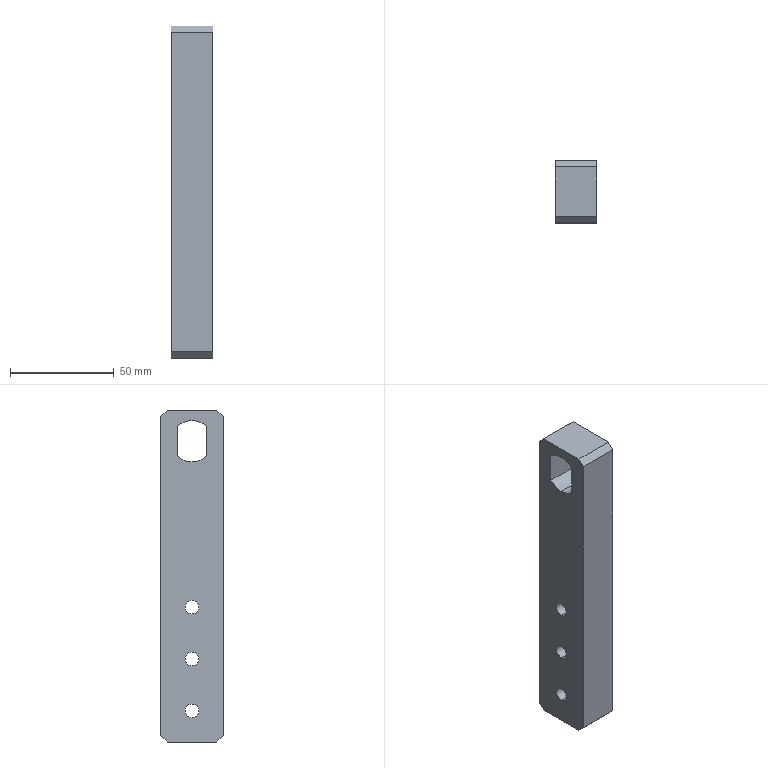Part | SolidWorks | features Chamfer 1, Extrusion 1, HoleWzd 1, ICE 1 | 1 solid | 30 faces | box 20 x 30 x 160 mm | volume 87200 mm3 | cylinder 15 | plane 15 | commonest cylinder face diameters 6.6 x6 11 x6 20 x3
STEP:
#1=CARTESIAN_POINT('',(13.2,0.,-9.5));
#2=VERTEX_POINT('',#1);
#3=CARTESIAN_POINT('',(13.2,0.,-20.5));
#4=VERTEX_POINT('',#3);
#5=CARTESIAN_POINT('',(13.2,0.,-15.));
#6=DIRECTION('',(1.,0.,0.));
#7=DIRECTION('',(0.,0.,-1.));
#8=AXIS2_PLACEMENT_3D('',#5,#6,#7);
#9=CIRCLE('',#8,5.5);
#10=EDGE_CURVE('',#2,#4,#9,.T.);
#11=ORIENTED_EDGE('',*,*,#10,.F.);
#12=CARTESIAN_POINT('',(20.,0.,-9.5));
#13=VERTEX_POINT('',#12);
#14=CARTESIAN_POINT('',(20.,0.,-9.5));
#15=DIRECTION('',(1.,0.,0.));
#16=VECTOR('',#15,1000.);
#17=LINE('',#14,#16);
#18=EDGE_CURVE('',#2,#13,#17,.T.);
#19=ORIENTED_EDGE('',*,*,#18,.T.);
#20=CARTESIAN_POINT('',(20.,0.,-20.5));
#21=VERTEX_POINT('',#20);
#22=CARTESIAN_POINT('',(20.,0.,-15.));
#23=DIRECTION('',(1.,0.,0.));
#24=DIRECTION('',(0.,0.,-1.));
#25=AXIS2_PLACEMENT_3D('',#22,#23,#24);
#26=CIRCLE('',#25,5.5);
#27=EDGE_CURVE('',#13,#21,#26,.T.);
#28=ORIENTED_EDGE('',*,*,#27,.T.);
#29=CARTESIAN_POINT('',(20.,0.,-20.5));
#30=DIRECTION('',(1.,0.,0.));
#31=VECTOR('',#30,1000.);
#32=LINE('',#29,#31);
#33=EDGE_CURVE('',#4,#21,#32,.T.);
#34=ORIENTED_EDGE('',*,*,#33,.F.);
#35=EDGE_LOOP('',(#11,#19,#28,#34));
#36=FACE_OUTER_BOUND('',#35,.T.);
#37=CARTESIAN_POINT('',(20.,0.,-15.));
#38=DIRECTION('',(1.,0.,0.));
#39=DIRECTION('',(0.,0.,-1.));
#40=AXIS2_PLACEMENT_3D('',#37,#38,#39);
#41=CYLINDRICAL_SURFACE('',#40,5.5);
#42=ADVANCED_FACE('',(#36),#41,.F.);
#43=CARTESIAN_POINT('',(0.,0.,-11.7));
#44=VERTEX_POINT('',#43);
#45=CARTESIAN_POINT('',(0.,0.,-18.3));
#46=VERTEX_POINT('',#45);
#47=CARTESIAN_POINT('',(0.,0.,-15.));
#48=DIRECTION('',(1.,0.,0.));
#49=DIRECTION('',(0.,0.,-1.));
#50=AXIS2_PLACEMENT_3D('',#47,#48,#49);
#51=CIRCLE('',#50,3.3);
#52=EDGE_CURVE('',#44,#46,#51,.T.);
#53=ORIENTED_EDGE('',*,*,#52,.F.);
#54=CARTESIAN_POINT('',(13.2,0.,-11.7));
#55=VERTEX_POINT('',#54);
#56=CARTESIAN_POINT('',(20.,0.,-11.7));
#57=DIRECTION('',(1.,0.,0.));
#58=VECTOR('',#57,1000.);
#59=LINE('',#56,#58);
#60=EDGE_CURVE('',#44,#55,#59,.T.);
#61=ORIENTED_EDGE('',*,*,#60,.T.);
#62=CARTESIAN_POINT('',(13.2,0.,-18.3));
#63=VERTEX_POINT('',#62);
#64=CARTESIAN_POINT('',(13.2,0.,-15.));
#65=DIRECTION('',(1.,0.,0.));
#66=DIRECTION('',(0.,0.,-1.));
#67=AXIS2_PLACEMENT_3D('',#64,#65,#66);
#68=CIRCLE('',#67,3.3);
#69=EDGE_CURVE('',#55,#63,#68,.T.);
#70=ORIENTED_EDGE('',*,*,#69,.T.);
#71=CARTESIAN_POINT('',(20.,0.,-18.3));
#72=DIRECTION('',(1.,0.,0.));
#73=VECTOR('',#72,1000.);
#74=LINE('',#71,#73);
#75=EDGE_CURVE('',#46,#63,#74,.T.);
#76=ORIENTED_EDGE('',*,*,#75,.F.);
#77=EDGE_LOOP('',(#53,#61,#70,#76));
#78=FACE_OUTER_BOUND('',#77,.T.);
#79=CARTESIAN_POINT('',(20.,0.,-15.));
#80=DIRECTION('',(1.,0.,0.));
#81=DIRECTION('',(0.,0.,-1.));
#82=AXIS2_PLACEMENT_3D('',#79,#80,#81);
#83=CYLINDRICAL_SURFACE('',#82,3.3);
#84=ADVANCED_FACE('',(#78),#83,.F.);
#85=CARTESIAN_POINT('',(13.2,0.,-34.5));
#86=VERTEX_POINT('',#85);
#87=CARTESIAN_POINT('',(13.2,0.,-45.5));
#88=VERTEX_POINT('',#87);
#89=CARTESIAN_POINT('',(13.2,0.,-40.));
#90=DIRECTION('',(1.,0.,0.));
#91=DIRECTION('',(0.,0.,-1.));
#92=AXIS2_PLACEMENT_3D('',#89,#90,#91);
#93=CIRCLE('',#92,5.5);
#94=EDGE_CURVE('',#86,#88,#93,.T.);
#95=ORIENTED_EDGE('',*,*,#94,.F.);
#96=CARTESIAN_POINT('',(20.,0.,-34.5));
#97=VERTEX_POINT('',#96);
#98=CARTESIAN_POINT('',(20.,0.,-34.5));
#99=DIRECTION('',(1.,0.,0.));
#100=VECTOR('',#99,1000.);
#101=LINE('',#98,#100);
#102=EDGE_CURVE('',#86,#97,#101,.T.);
#103=ORIENTED_EDGE('',*,*,#102,.T.);
#104=CARTESIAN_POINT('',(20.,0.,-45.5));
#105=VERTEX_POINT('',#104);
#106=CARTESIAN_POINT('',(20.,0.,-40.));
#107=DIRECTION('',(1.,0.,0.));
#108=DIRECTION('',(0.,0.,-1.));
#109=AXIS2_PLACEMENT_3D('',#106,#107,#108);
#110=CIRCLE('',#109,5.5);
#111=EDGE_CURVE('',#97,#105,#110,.T.);
#112=ORIENTED_EDGE('',*,*,#111,.T.);
#113=CARTESIAN_POINT('',(20.,0.,-45.5));
#114=DIRECTION('',(1.,0.,0.));
#115=VECTOR('',#114,1000.);
#116=LINE('',#113,#115);
#117=EDGE_CURVE('',#88,#105,#116,.T.);
#118=ORIENTED_EDGE('',*,*,#117,.F.);
#119=EDGE_LOOP('',(#95,#103,#112,#118));
#120=FACE_OUTER_BOUND('',#119,.T.);
#121=CARTESIAN_POINT('',(20.,0.,-40.));
#122=DIRECTION('',(1.,0.,0.));
#123=DIRECTION('',(0.,0.,-1.));
#124=AXIS2_PLACEMENT_3D('',#121,#122,#123);
#125=CYLINDRICAL_SURFACE('',#124,5.5);
#126=ADVANCED_FACE('',(#120),#125,.F.);
#127=CARTESIAN_POINT('',(0.,0.,-36.7));
#128=VERTEX_POINT('',#127);
#129=CARTESIAN_POINT('',(0.,0.,-43.3));
#130=VERTEX_POINT('',#129);
#131=CARTESIAN_POINT('',(0.,0.,-40.));
#132=DIRECTION('',(1.,0.,0.));
#133=DIRECTION('',(0.,0.,-1.));
#134=AXIS2_PLACEMENT_3D('',#131,#132,#133);
#135=CIRCLE('',#134,3.3);
#136=EDGE_CURVE('',#128,#130,#135,.T.);
#137=ORIENTED_EDGE('',*,*,#136,.F.);
#138=CARTESIAN_POINT('',(13.2,0.,-36.7));
#139=VERTEX_POINT('',#138);
#140=CARTESIAN_POINT('',(20.,0.,-36.7));
#141=DIRECTION('',(1.,0.,0.));
#142=VECTOR('',#141,1000.);
#143=LINE('',#140,#142);
#144=EDGE_CURVE('',#128,#139,#143,.T.);
#145=ORIENTED_EDGE('',*,*,#144,.T.);
#146=CARTESIAN_POINT('',(13.2,0.,-43.3));
#147=VERTEX_POINT('',#146);
#148=CARTESIAN_POINT('',(13.2,0.,-40.));
#149=DIRECTION('',(1.,0.,0.));
#150=DIRECTION('',(0.,0.,-1.));
#151=AXIS2_PLACEMENT_3D('',#148,#149,#150);
#152=CIRCLE('',#151,3.3);
#153=EDGE_CURVE('',#139,#147,#152,.T.);
#154=ORIENTED_EDGE('',*,*,#153,.T.);
#155=CARTESIAN_POINT('',(20.,0.,-43.3));
#156=DIRECTION('',(1.,0.,0.));
#157=VECTOR('',#156,1000.);
#158=LINE('',#155,#157);
#159=EDGE_CURVE('',#130,#147,#158,.T.);
#160=ORIENTED_EDGE('',*,*,#159,.F.);
#161=EDGE_LOOP('',(#137,#145,#154,#160));
#162=FACE_OUTER_BOUND('',#161,.T.);
#163=CARTESIAN_POINT('',(20.,0.,-40.));
#164=DIRECTION('',(1.,0.,0.));
#165=DIRECTION('',(0.,0.,-1.));
#166=AXIS2_PLACEMENT_3D('',#163,#164,#165);
#167=CYLINDRICAL_SURFACE('',#166,3.3);
#168=ADVANCED_FACE('',(#162),#167,.F.);
#169=CARTESIAN_POINT('',(13.2,0.,-59.5));
#170=VERTEX_POINT('',#169);
#171=CARTESIAN_POINT('',(13.2,0.,-70.5));
#172=VERTEX_POINT('',#171);
#173=CARTESIAN_POINT('',(13.2,0.,-65.));
#174=DIRECTION('',(1.,0.,0.));
#175=DIRECTION('',(0.,0.,-1.));
#176=AXIS2_PLACEMENT_3D('',#173,#174,#175);
#177=CIRCLE('',#176,5.5);
#178=EDGE_CURVE('',#170,#172,#177,.T.);
#179=ORIENTED_EDGE('',*,*,#178,.F.);
#180=CARTESIAN_POINT('',(20.,0.,-59.5));
#181=VERTEX_POINT('',#180);
#182=CARTESIAN_POINT('',(20.,0.,-59.5));
#183=DIRECTION('',(1.,0.,0.));
#184=VECTOR('',#183,1000.);
#185=LINE('',#182,#184);
#186=EDGE_CURVE('',#170,#181,#185,.T.);
#187=ORIENTED_EDGE('',*,*,#186,.T.);
#188=CARTESIAN_POINT('',(20.,0.,-70.5));
#189=VERTEX_POINT('',#188);
#190=CARTESIAN_POINT('',(20.,0.,-65.));
#191=DIRECTION('',(1.,0.,0.));
#192=DIRECTION('',(0.,0.,-1.));
#193=AXIS2_PLACEMENT_3D('',#190,#191,#192);
#194=CIRCLE('',#193,5.5);
#195=EDGE_CURVE('',#181,#189,#194,.T.);
#196=ORIENTED_EDGE('',*,*,#195,.T.);
#197=CARTESIAN_POINT('',(20.,0.,-70.5));
#198=DIRECTION('',(1.,0.,0.));
#199=VECTOR('',#198,1000.);
#200=LINE('',#197,#199);
#201=EDGE_CURVE('',#172,#189,#200,.T.);
#202=ORIENTED_EDGE('',*,*,#201,.F.);
#203=EDGE_LOOP('',(#179,#187,#196,#202));
#204=FACE_OUTER_BOUND('',#203,.T.);
#205=CARTESIAN_POINT('',(20.,0.,-65.));
#206=DIRECTION('',(1.,0.,0.));
#207=DIRECTION('',(0.,0.,-1.));
#208=AXIS2_PLACEMENT_3D('',#205,#206,#207);
#209=CYLINDRICAL_SURFACE('',#208,5.5);
#210=ADVANCED_FACE('',(#204),#209,.F.);
#211=CARTESIAN_POINT('',(0.,0.,-61.7));
#212=VERTEX_POINT('',#211);
#213=CARTESIAN_POINT('',(0.,0.,-68.3));
#214=VERTEX_POINT('',#213);
#215=CARTESIAN_POINT('',(0.,0.,-65.));
#216=DIRECTION('',(1.,0.,0.));
#217=DIRECTION('',(0.,0.,-1.));
#218=AXIS2_PLACEMENT_3D('',#215,#216,#217);
#219=CIRCLE('',#218,3.3);
#220=EDGE_CURVE('',#212,#214,#219,.T.);
#221=ORIENTED_EDGE('',*,*,#220,.F.);
#222=CARTESIAN_POINT('',(13.2,0.,-61.7));
#223=VERTEX_POINT('',#222);
#224=CARTESIAN_POINT('',(20.,0.,-61.7));
#225=DIRECTION('',(1.,0.,0.));
#226=VECTOR('',#225,1000.);
#227=LINE('',#224,#226);
#228=EDGE_CURVE('',#212,#223,#227,.T.);
#229=ORIENTED_EDGE('',*,*,#228,.T.);
#230=CARTESIAN_POINT('',(13.2,0.,-68.3));
#231=VERTEX_POINT('',#230);
#232=CARTESIAN_POINT('',(13.2,0.,-65.));
#233=DIRECTION('',(1.,0.,0.));
#234=DIRECTION('',(0.,0.,-1.));
#235=AXIS2_PLACEMENT_3D('',#232,#233,#234);
#236=CIRCLE('',#235,3.3);
#237=EDGE_CURVE('',#223,#231,#236,.T.);
#238=ORIENTED_EDGE('',*,*,#237,.T.);
#239=CARTESIAN_POINT('',(20.,0.,-68.3));
#240=DIRECTION('',(1.,0.,0.));
#241=VECTOR('',#240,1000.);
#242=LINE('',#239,#241);
#243=EDGE_CURVE('',#214,#231,#242,.T.);
#244=ORIENTED_EDGE('',*,*,#243,.F.);
#245=EDGE_LOOP('',(#221,#229,#238,#244));
#246=FACE_OUTER_BOUND('',#245,.T.);
#247=CARTESIAN_POINT('',(20.,0.,-65.));
#248=DIRECTION('',(1.,0.,0.));
#249=DIRECTION('',(0.,0.,-1.));
#250=AXIS2_PLACEMENT_3D('',#247,#248,#249);
#251=CYLINDRICAL_SURFACE('',#250,3.3);
#252=ADVANCED_FACE('',(#246),#251,.F.);
#253=CARTESIAN_POINT('',(0.,0.,55.));
#254=VERTEX_POINT('',#253);
#255=CARTESIAN_POINT('',(0.,7.08,57.938));
#256=VERTEX_POINT('',#255);
#257=CARTESIAN_POINT('',(0.,0.,65.));
#258=DIRECTION('',(1.,0.,0.));
#259=DIRECTION('',(0.,0.,-1.));
#260=AXIS2_PLACEMENT_3D('',#257,#258,#259);
#261=CIRCLE('',#260,10.);
#262=EDGE_CURVE('',#254,#256,#261,.T.);
#263=ORIENTED_EDGE('',*,*,#262,.F.);
#264=CARTESIAN_POINT('',(20.,0.,55.));
#265=VERTEX_POINT('',#264);
#266=CARTESIAN_POINT('',(0.,0.,55.));
#267=DIRECTION('',(1.,0.,0.));
#268=VECTOR('',#267,1000.);
#269=LINE('',#266,#268);
#270=EDGE_CURVE('',#254,#265,#269,.T.);
#271=ORIENTED_EDGE('',*,*,#270,.T.);
#272=CARTESIAN_POINT('',(20.,7.08,57.938));
#273=VERTEX_POINT('',#272);
#274=CARTESIAN_POINT('',(20.,0.,65.));
#275=DIRECTION('',(1.,0.,0.));
#276=DIRECTION('',(0.,0.,-1.));
#277=AXIS2_PLACEMENT_3D('',#274,#275,#276);
#278=CIRCLE('',#277,10.);
#279=EDGE_CURVE('',#265,#273,#278,.T.);
#280=ORIENTED_EDGE('',*,*,#279,.T.);
#281=CARTESIAN_POINT('',(0.,7.08,57.938));
#282=DIRECTION('',(1.,0.,0.));
#283=VECTOR('',#282,1000.);
#284=LINE('',#281,#283);
#285=EDGE_CURVE('',#256,#273,#284,.T.);
#286=ORIENTED_EDGE('',*,*,#285,.F.);
#287=EDGE_LOOP('',(#263,#271,#280,#286));
#288=FACE_OUTER_BOUND('',#287,.T.);
#289=CARTESIAN_POINT('',(0.,0.,65.));
#290=DIRECTION('',(1.,0.,0.));
#291=DIRECTION('',(0.,0.,-1.));
#292=AXIS2_PLACEMENT_3D('',#289,#290,#291);
#293=CYLINDRICAL_SURFACE('',#292,10.);
#294=ADVANCED_FACE('',(#288),#293,.F.);
#295=CARTESIAN_POINT('',(0.,-12.,-80.));
#296=VERTEX_POINT('',#295);
#297=CARTESIAN_POINT('',(0.,12.,-80.));
#298=VERTEX_POINT('',#297);
#299=CARTESIAN_POINT('',(0.,15.,-80.));
#300=DIRECTION('',(0.,1.,0.));
#301=VECTOR('',#300,1000.);
#302=LINE('',#299,#301);
#303=EDGE_CURVE('',#296,#298,#302,.T.);
#304=ORIENTED_EDGE('',*,*,#303,.T.);
#305=CARTESIAN_POINT('',(20.,12.,-80.));
#306=VERTEX_POINT('',#305);
#307=CARTESIAN_POINT('',(20.,12.,-80.));
#308=DIRECTION('',(1.,0.,0.));
#309=VECTOR('',#308,1000.);
#310=LINE('',#307,#309);
#311=EDGE_CURVE('',#298,#306,#310,.T.);
#312=ORIENTED_EDGE('',*,*,#311,.T.);
#313=CARTESIAN_POINT('',(20.,-12.,-80.));
#314=VERTEX_POINT('',#313);
#315=CARTESIAN_POINT('',(20.,15.,-80.));
#316=DIRECTION('',(0.,1.,0.));
#317=VECTOR('',#316,1000.);
#318=LINE('',#315,#317);
#319=EDGE_CURVE('',#314,#306,#318,.T.);
#320=ORIENTED_EDGE('',*,*,#319,.F.);
#321=CARTESIAN_POINT('',(20.,-12.,-80.));
#322=DIRECTION('',(-1.,0.,0.));
#323=VECTOR('',#322,1000.);
#324=LINE('',#321,#323);
#325=EDGE_CURVE('',#314,#296,#324,.T.);
#326=ORIENTED_EDGE('',*,*,#325,.T.);
#327=EDGE_LOOP('',(#304,#312,#320,#326));
#328=FACE_OUTER_BOUND('',#327,.T.);
#329=CARTESIAN_POINT('',(20.,15.,-80.));
#330=DIRECTION('',(0.,0.,1.));
#331=DIRECTION('',(1.,0.,0.));
#332=AXIS2_PLACEMENT_3D('',#329,#330,#331);
#333=PLANE('',#332);
#334=ADVANCED_FACE('',(#328),#333,.F.);
#335=CARTESIAN_POINT('',(0.,15.,-77.));
#336=VERTEX_POINT('',#335);
#337=CARTESIAN_POINT('',(0.,15.,77.));
#338=VERTEX_POINT('',#337);
#339=CARTESIAN_POINT('',(0.,15.,80.));
#340=DIRECTION('',(0.,0.,1.));
#341=VECTOR('',#340,1000.);
#342=LINE('',#339,#341);
#343=EDGE_CURVE('',#336,#338,#342,.T.);
#344=ORIENTED_EDGE('',*,*,#343,.T.);
#345=CARTESIAN_POINT('',(20.,15.,77.));
#346=VERTEX_POINT('',#345);
#347=CARTESIAN_POINT('',(20.,15.,77.));
#348=DIRECTION('',(1.,0.,0.));
#349=VECTOR('',#348,1000.);
#350=LINE('',#347,#349);
#351=EDGE_CURVE('',#338,#346,#350,.T.);
#352=ORIENTED_EDGE('',*,*,#351,.T.);
#353=CARTESIAN_POINT('',(20.,15.,-77.));
#354=VERTEX_POINT('',#353);
#355=CARTESIAN_POINT('',(20.,15.,80.));
#356=DIRECTION('',(0.,0.,1.));
#357=VECTOR('',#356,1000.);
#358=LINE('',#355,#357);
#359=EDGE_CURVE('',#354,#346,#358,.T.);
#360=ORIENTED_EDGE('',*,*,#359,.F.);
#361=CARTESIAN_POINT('',(20.,15.,-77.));
#362=DIRECTION('',(-1.,0.,0.));
#363=VECTOR('',#362,1000.);
#364=LINE('',#361,#363);
#365=EDGE_CURVE('',#354,#336,#364,.T.);
#366=ORIENTED_EDGE('',*,*,#365,.T.);
#367=EDGE_LOOP('',(#344,#352,#360,#366));
#368=FACE_OUTER_BOUND('',#367,.T.);
#369=CARTESIAN_POINT('',(20.,15.,80.));
#370=DIRECTION('',(0.,-1.,0.));
#371=DIRECTION('',(0.,0.,-1.));
#372=AXIS2_PLACEMENT_3D('',#369,#370,#371);
#373=PLANE('',#372);
#374=ADVANCED_FACE('',(#368),#373,.F.);
#375=CARTESIAN_POINT('',(20.,12.,80.));
#376=VERTEX_POINT('',#375);
#377=CARTESIAN_POINT('',(20.,-12.,80.));
#378=VERTEX_POINT('',#377);
#379=CARTESIAN_POINT('',(20.,15.,80.));
#380=DIRECTION('',(0.,-1.,0.));
#381=VECTOR('',#380,1000.);
#382=LINE('',#379,#381);
#383=EDGE_CURVE('',#376,#378,#382,.T.);
#384=ORIENTED_EDGE('',*,*,#383,.F.);
#385=CARTESIAN_POINT('',(0.,12.,80.));
#386=VERTEX_POINT('',#385);
#387=CARTESIAN_POINT('',(20.,12.,80.));
#388=DIRECTION('',(-1.,0.,0.));
#389=VECTOR('',#388,1000.);
#390=LINE('',#387,#389);
#391=EDGE_CURVE('',#376,#386,#390,.T.);
#392=ORIENTED_EDGE('',*,*,#391,.T.);
#393=CARTESIAN_POINT('',(0.,-12.,80.));
#394=VERTEX_POINT('',#393);
#395=CARTESIAN_POINT('',(0.,15.,80.));
#396=DIRECTION('',(0.,-1.,0.));
#397=VECTOR('',#396,1000.);
#398=LINE('',#395,#397);
#399=EDGE_CURVE('',#386,#394,#398,.T.);
#400=ORIENTED_EDGE('',*,*,#399,.T.);
#401=CARTESIAN_POINT('',(20.,-12.,80.));
#402=DIRECTION('',(1.,0.,0.));
#403=VECTOR('',#402,1000.);
#404=LINE('',#401,#403);
#405=EDGE_CURVE('',#394,#378,#404,.T.);
#406=ORIENTED_EDGE('',*,*,#405,.T.);
#407=EDGE_LOOP('',(#384,#392,#400,#406));
#408=FACE_OUTER_BOUND('',#407,.T.);
#409=CARTESIAN_POINT('',(20.,15.,80.));
#410=DIRECTION('',(0.,0.,-1.));
#411=DIRECTION('',(-1.,0.,0.));
#412=AXIS2_PLACEMENT_3D('',#409,#410,#411);
#413=PLANE('',#412);
#414=ADVANCED_FACE('',(#408),#413,.F.);
#415=CARTESIAN_POINT('',(20.,-15.,77.));
#416=VERTEX_POINT('',#415);
#417=CARTESIAN_POINT('',(20.,-15.,-77.));
#418=VERTEX_POINT('',#417);
#419=CARTESIAN_POINT('',(20.,-15.,80.));
#420=DIRECTION('',(0.,0.,-1.));
#421=VECTOR('',#420,1000.);
#422=LINE('',#419,#421);
#423=EDGE_CURVE('',#416,#418,#422,.T.);
#424=ORIENTED_EDGE('',*,*,#423,.F.);
#425=CARTESIAN_POINT('',(0.,-15.,77.));
#426=VERTEX_POINT('',#425);
#427=CARTESIAN_POINT('',(20.,-15.,77.));
#428=DIRECTION('',(-1.,0.,0.));
#429=VECTOR('',#428,1000.);
#430=LINE('',#427,#429);
#431=EDGE_CURVE('',#416,#426,#430,.T.);
#432=ORIENTED_EDGE('',*,*,#431,.T.);
#433=CARTESIAN_POINT('',(0.,-15.,-77.));
#434=VERTEX_POINT('',#433);
#435=CARTESIAN_POINT('',(0.,-15.,80.));
#436=DIRECTION('',(0.,0.,-1.));
#437=VECTOR('',#436,1000.);
#438=LINE('',#435,#437);
#439=EDGE_CURVE('',#426,#434,#438,.T.);
#440=ORIENTED_EDGE('',*,*,#439,.T.);
#441=CARTESIAN_POINT('',(20.,-15.,-77.));
#442=DIRECTION('',(1.,0.,0.));
#443=VECTOR('',#442,1000.);
#444=LINE('',#441,#443);
#445=EDGE_CURVE('',#434,#418,#444,.T.);
#446=ORIENTED_EDGE('',*,*,#445,.T.);
#447=EDGE_LOOP('',(#424,#432,#440,#446));
#448=FACE_OUTER_BOUND('',#447,.T.);
#449=CARTESIAN_POINT('',(20.,-15.,80.));
#450=DIRECTION('',(0.,1.,0.));
#451=DIRECTION('',(0.,0.,1.));
#452=AXIS2_PLACEMENT_3D('',#449,#450,#451);
#453=PLANE('',#452);
#454=ADVANCED_FACE('',(#448),#453,.F.);
#455=CARTESIAN_POINT('',(20.,0.,-15.));
#456=DIRECTION('',(1.,0.,0.));
#457=DIRECTION('',(0.,0.,-1.));
#458=AXIS2_PLACEMENT_3D('',#455,#456,#457);
#459=CIRCLE('',#458,5.5);
#460=EDGE_CURVE('',#21,#13,#459,.T.);
#461=ORIENTED_EDGE('',*,*,#460,.F.);
#462=ORIENTED_EDGE('',*,*,#27,.F.);
#463=EDGE_LOOP('',(#461,#462));
#464=FACE_BOUND('',#463,.T.);
#465=CARTESIAN_POINT('',(20.,0.,-40.));
#466=DIRECTION('',(1.,0.,0.));
#467=DIRECTION('',(0.,0.,-1.));
#468=AXIS2_PLACEMENT_3D('',#465,#466,#467);
#469=CIRCLE('',#468,5.5);
#470=EDGE_CURVE('',#105,#97,#469,.T.);
#471=ORIENTED_EDGE('',*,*,#470,.F.);
#472=ORIENTED_EDGE('',*,*,#111,.F.);
#473=EDGE_LOOP('',(#471,#472));
#474=FACE_BOUND('',#473,.T.);
#475=CARTESIAN_POINT('',(20.,0.,-65.));
#476=DIRECTION('',(1.,0.,0.));
#477=DIRECTION('',(0.,0.,-1.));
#478=AXIS2_PLACEMENT_3D('',#475,#476,#477);
#479=CIRCLE('',#478,5.5);
#480=EDGE_CURVE('',#189,#181,#479,.T.);
#481=ORIENTED_EDGE('',*,*,#480,.F.);
#482=ORIENTED_EDGE('',*,*,#195,.F.);
#483=EDGE_LOOP('',(#481,#482));
#484=FACE_BOUND('',#483,.T.);
#485=CARTESIAN_POINT('',(20.,-7.08,57.938));
#486=VERTEX_POINT('',#485);
#487=CARTESIAN_POINT('',(20.,0.,65.));
#488=DIRECTION('',(1.,0.,0.));
#489=DIRECTION('',(0.,0.,-1.));
#490=AXIS2_PLACEMENT_3D('',#487,#488,#489);
#491=CIRCLE('',#490,10.);
#492=EDGE_CURVE('',#486,#265,#491,.T.);
#493=ORIENTED_EDGE('',*,*,#492,.F.);
#494=CARTESIAN_POINT('',(20.,-7.08,72.062));
#495=VERTEX_POINT('',#494);
#496=CARTESIAN_POINT('',(20.,-7.08,72.062));
#497=DIRECTION('',(0.,0.,-1.));
#498=VECTOR('',#497,1000.);
#499=LINE('',#496,#498);
#500=EDGE_CURVE('',#495,#486,#499,.T.);
#501=ORIENTED_EDGE('',*,*,#500,.F.);
#502=CARTESIAN_POINT('',(20.,7.08,72.062));
#503=VERTEX_POINT('',#502);
#504=CARTESIAN_POINT('',(20.,0.,65.));
#505=DIRECTION('',(1.,0.,0.));
#506=DIRECTION('',(0.,0.,-1.));
#507=AXIS2_PLACEMENT_3D('',#504,#505,#506);
#508=CIRCLE('',#507,10.);
#509=EDGE_CURVE('',#503,#495,#508,.T.);
#510=ORIENTED_EDGE('',*,*,#509,.F.);
#511=CARTESIAN_POINT('',(20.,7.08,72.062));
#512=DIRECTION('',(0.,0.,1.));
#513=VECTOR('',#512,1000.);
#514=LINE('',#511,#513);
#515=EDGE_CURVE('',#273,#503,#514,.T.);
#516=ORIENTED_EDGE('',*,*,#515,.F.);
#517=ORIENTED_EDGE('',*,*,#279,.F.);
#518=EDGE_LOOP('',(#493,#501,#510,#516,#517));
#519=FACE_BOUND('',#518,.T.);
#520=ORIENTED_EDGE('',*,*,#359,.T.);
#521=CARTESIAN_POINT('',(20.,46.,46.));
#522=DIRECTION('',(0.,-0.7071,0.7071));
#523=VECTOR('',#522,1000.);
#524=LINE('',#521,#523);
#525=EDGE_CURVE('',#346,#376,#524,.T.);
#526=ORIENTED_EDGE('',*,*,#525,.T.);
#527=ORIENTED_EDGE('',*,*,#383,.T.);
#528=CARTESIAN_POINT('',(20.,-46.,46.));
#529=DIRECTION('',(0.,-0.7071,-0.7071));
#530=VECTOR('',#529,1000.);
#531=LINE('',#528,#530);
#532=EDGE_CURVE('',#378,#416,#531,.T.);
#533=ORIENTED_EDGE('',*,*,#532,.T.);
#534=ORIENTED_EDGE('',*,*,#423,.T.);
#535=CARTESIAN_POINT('',(20.,-46.,-46.));
#536=DIRECTION('',(0.,0.7071,-0.7071));
#537=VECTOR('',#536,1000.);
#538=LINE('',#535,#537);
#539=EDGE_CURVE('',#418,#314,#538,.T.);
#540=ORIENTED_EDGE('',*,*,#539,.T.);
#541=ORIENTED_EDGE('',*,*,#319,.T.);
#542=CARTESIAN_POINT('',(20.,46.,-46.));
#543=DIRECTION('',(0.,0.7071,0.7071));
#544=VECTOR('',#543,1000.);
#545=LINE('',#542,#544);
#546=EDGE_CURVE('',#306,#354,#545,.T.);
#547=ORIENTED_EDGE('',*,*,#546,.T.);
#548=EDGE_LOOP('',(#520,#526,#527,#533,#534,#540,#541,#547));
#549=FACE_OUTER_BOUND('',#548,.T.);
#550=CARTESIAN_POINT('',(20.,0.,0.));
#551=DIRECTION('',(1.,0.,0.));
#552=DIRECTION('',(0.,0.,-1.));
#553=AXIS2_PLACEMENT_3D('',#550,#551,#552);
#554=PLANE('',#553);
#555=ADVANCED_FACE('',(#464,#474,#484,#519,#549),#554,.T.);
#556=CARTESIAN_POINT('',(0.,0.,-15.));
#557=DIRECTION('',(1.,0.,0.));
#558=DIRECTION('',(0.,0.,-1.));
#559=AXIS2_PLACEMENT_3D('',#556,#557,#558);
#560=CIRCLE('',#559,3.3);
#561=EDGE_CURVE('',#46,#44,#560,.T.);
#562=ORIENTED_EDGE('',*,*,#561,.T.);
#563=ORIENTED_EDGE('',*,*,#52,.T.);
#564=EDGE_LOOP('',(#562,#563));
#565=FACE_BOUND('',#564,.T.);
#566=CARTESIAN_POINT('',(0.,0.,-40.));
#567=DIRECTION('',(1.,0.,0.));
#568=DIRECTION('',(0.,0.,-1.));
#569=AXIS2_PLACEMENT_3D('',#566,#567,#568);
#570=CIRCLE('',#569,3.3);
#571=EDGE_CURVE('',#130,#128,#570,.T.);
#572=ORIENTED_EDGE('',*,*,#571,.T.);
#573=ORIENTED_EDGE('',*,*,#136,.T.);
#574=EDGE_LOOP('',(#572,#573));
#575=FACE_BOUND('',#574,.T.);
#576=CARTESIAN_POINT('',(0.,0.,-65.));
#577=DIRECTION('',(1.,0.,0.));
#578=DIRECTION('',(0.,0.,-1.));
#579=AXIS2_PLACEMENT_3D('',#576,#577,#578);
#580=CIRCLE('',#579,3.3);
#581=EDGE_CURVE('',#214,#212,#580,.T.);
#582=ORIENTED_EDGE('',*,*,#581,.T.);
#583=ORIENTED_EDGE('',*,*,#220,.T.);
#584=EDGE_LOOP('',(#582,#583));
#585=FACE_BOUND('',#584,.T.);
#586=CARTESIAN_POINT('',(0.,-7.08,72.062));
#587=VERTEX_POINT('',#586);
#588=CARTESIAN_POINT('',(0.,-7.08,57.938));
#589=VERTEX_POINT('',#588);
#590=CARTESIAN_POINT('',(0.,-7.08,72.062));
#591=DIRECTION('',(0.,0.,-1.));
#592=VECTOR('',#591,1000.);
#593=LINE('',#590,#592);
#594=EDGE_CURVE('',#587,#589,#593,.T.);
#595=ORIENTED_EDGE('',*,*,#594,.T.);
#596=CARTESIAN_POINT('',(0.,0.,65.));
#597=DIRECTION('',(1.,0.,0.));
#598=DIRECTION('',(0.,0.,-1.));
#599=AXIS2_PLACEMENT_3D('',#596,#597,#598);
#600=CIRCLE('',#599,10.);
#601=EDGE_CURVE('',#589,#254,#600,.T.);
#602=ORIENTED_EDGE('',*,*,#601,.T.);
#603=ORIENTED_EDGE('',*,*,#262,.T.);
#604=CARTESIAN_POINT('',(0.,7.08,72.062));
#605=VERTEX_POINT('',#604);
#606=CARTESIAN_POINT('',(0.,7.08,72.062));
#607=DIRECTION('',(0.,0.,1.));
#608=VECTOR('',#607,1000.);
#609=LINE('',#606,#608);
#610=EDGE_CURVE('',#256,#605,#609,.T.);
#611=ORIENTED_EDGE('',*,*,#610,.T.);
#612=CARTESIAN_POINT('',(0.,0.,65.));
#613=DIRECTION('',(1.,0.,0.));
#614=DIRECTION('',(0.,0.,-1.));
#615=AXIS2_PLACEMENT_3D('',#612,#613,#614);
#616=CIRCLE('',#615,10.);
#617=EDGE_CURVE('',#605,#587,#616,.T.);
#618=ORIENTED_EDGE('',*,*,#617,.T.);
#619=EDGE_LOOP('',(#595,#602,#603,#611,#618));
#620=FACE_BOUND('',#619,.T.);
#621=ORIENTED_EDGE('',*,*,#399,.F.);
#622=CARTESIAN_POINT('',(0.,12.,80.));
#623=DIRECTION('',(0.,0.7071,-0.7071));
#624=VECTOR('',#623,1000.);
#625=LINE('',#622,#624);
#626=EDGE_CURVE('',#386,#338,#625,.T.);
#627=ORIENTED_EDGE('',*,*,#626,.T.);
#628=ORIENTED_EDGE('',*,*,#343,.F.);
#629=CARTESIAN_POINT('',(0.,15.,-77.));
#630=DIRECTION('',(0.,-0.7071,-0.7071));
#631=VECTOR('',#630,1000.);
#632=LINE('',#629,#631);
#633=EDGE_CURVE('',#336,#298,#632,.T.);
#634=ORIENTED_EDGE('',*,*,#633,.T.);
#635=ORIENTED_EDGE('',*,*,#303,.F.);
#636=CARTESIAN_POINT('',(0.,-12.,-80.));
#637=DIRECTION('',(0.,-0.7071,0.7071));
#638=VECTOR('',#637,1000.);
#639=LINE('',#636,#638);
#640=EDGE_CURVE('',#296,#434,#639,.T.);
#641=ORIENTED_EDGE('',*,*,#640,.T.);
#642=ORIENTED_EDGE('',*,*,#439,.F.);
#643=CARTESIAN_POINT('',(0.,-15.,77.));
#644=DIRECTION('',(0.,0.7071,0.7071));
#645=VECTOR('',#644,1000.);
#646=LINE('',#643,#645);
#647=EDGE_CURVE('',#426,#394,#646,.T.);
#648=ORIENTED_EDGE('',*,*,#647,.T.);
#649=EDGE_LOOP('',(#621,#627,#628,#634,#635,#641,#642,#648));
#650=FACE_OUTER_BOUND('',#649,.T.);
#651=CARTESIAN_POINT('',(0.,0.,0.));
#652=DIRECTION('',(1.,0.,0.));
#653=DIRECTION('',(0.,0.,-1.));
#654=AXIS2_PLACEMENT_3D('',#651,#652,#653);
#655=PLANE('',#654);
#656=ADVANCED_FACE('',(#565,#575,#585,#620,#650),#655,.F.);
#657=ORIENTED_EDGE('',*,*,#270,.F.);
#658=ORIENTED_EDGE('',*,*,#601,.F.);
#659=CARTESIAN_POINT('',(0.,-7.08,57.938));
#660=DIRECTION('',(1.,0.,0.));
#661=VECTOR('',#660,1000.);
#662=LINE('',#659,#661);
#663=EDGE_CURVE('',#589,#486,#662,.T.);
#664=ORIENTED_EDGE('',*,*,#663,.T.);
#665=ORIENTED_EDGE('',*,*,#492,.T.);
#666=EDGE_LOOP('',(#657,#658,#664,#665));
#667=FACE_OUTER_BOUND('',#666,.T.);
#668=CARTESIAN_POINT('',(0.,0.,65.));
#669=DIRECTION('',(1.,0.,0.));
#670=DIRECTION('',(0.,0.,-1.));
#671=AXIS2_PLACEMENT_3D('',#668,#669,#670);
#672=CYLINDRICAL_SURFACE('',#671,10.);
#673=ADVANCED_FACE('',(#667),#672,.F.);
#674=ORIENTED_EDGE('',*,*,#500,.T.);
#675=ORIENTED_EDGE('',*,*,#663,.F.);
#676=ORIENTED_EDGE('',*,*,#594,.F.);
#677=CARTESIAN_POINT('',(0.,-7.08,72.062));
#678=DIRECTION('',(1.,0.,0.));
#679=VECTOR('',#678,1000.);
#680=LINE('',#677,#679);
#681=EDGE_CURVE('',#587,#495,#680,.T.);
#682=ORIENTED_EDGE('',*,*,#681,.T.);
#683=EDGE_LOOP('',(#674,#675,#676,#682));
#684=FACE_OUTER_BOUND('',#683,.T.);
#685=CARTESIAN_POINT('',(0.,-7.08,72.062));
#686=DIRECTION('',(0.,-1.,0.));
#687=DIRECTION('',(0.,0.,-1.));
#688=AXIS2_PLACEMENT_3D('',#685,#686,#687);
#689=PLANE('',#688);
#690=ADVANCED_FACE('',(#684),#689,.F.);
#691=ORIENTED_EDGE('',*,*,#509,.T.);
#692=ORIENTED_EDGE('',*,*,#681,.F.);
#693=ORIENTED_EDGE('',*,*,#617,.F.);
#694=CARTESIAN_POINT('',(0.,7.08,72.062));
#695=DIRECTION('',(1.,0.,0.));
#696=VECTOR('',#695,1000.);
#697=LINE('',#694,#696);
#698=EDGE_CURVE('',#605,#503,#697,.T.);
#699=ORIENTED_EDGE('',*,*,#698,.T.);
#700=EDGE_LOOP('',(#691,#692,#693,#699));
#701=FACE_OUTER_BOUND('',#700,.T.);
#702=CARTESIAN_POINT('',(0.,0.,65.));
#703=DIRECTION('',(1.,0.,0.));
#704=DIRECTION('',(0.,0.,-1.));
#705=AXIS2_PLACEMENT_3D('',#702,#703,#704);
#706=CYLINDRICAL_SURFACE('',#705,10.);
#707=ADVANCED_FACE('',(#701),#706,.F.);
#708=ORIENTED_EDGE('',*,*,#515,.T.);
#709=ORIENTED_EDGE('',*,*,#698,.F.);
#710=ORIENTED_EDGE('',*,*,#610,.F.);
#711=ORIENTED_EDGE('',*,*,#285,.T.);
#712=EDGE_LOOP('',(#708,#709,#710,#711));
#713=FACE_OUTER_BOUND('',#712,.T.);
#714=CARTESIAN_POINT('',(0.,7.08,72.062));
#715=DIRECTION('',(0.,1.,0.));
#716=DIRECTION('',(0.,0.,1.));
#717=AXIS2_PLACEMENT_3D('',#714,#715,#716);
#718=PLANE('',#717);
#719=ADVANCED_FACE('',(#713),#718,.F.);
#720=ORIENTED_EDGE('',*,*,#228,.F.);
#721=ORIENTED_EDGE('',*,*,#581,.F.);
#722=ORIENTED_EDGE('',*,*,#243,.T.);
#723=CARTESIAN_POINT('',(13.2,0.,-65.));
#724=DIRECTION('',(1.,0.,0.));
#725=DIRECTION('',(0.,0.,-1.));
#726=AXIS2_PLACEMENT_3D('',#723,#724,#725);
#727=CIRCLE('',#726,3.3);
#728=EDGE_CURVE('',#231,#223,#727,.T.);
#729=ORIENTED_EDGE('',*,*,#728,.T.);
#730=EDGE_LOOP('',(#720,#721,#722,#729));
#731=FACE_OUTER_BOUND('',#730,.T.);
#732=CARTESIAN_POINT('',(20.,0.,-65.));
#733=DIRECTION('',(1.,0.,0.));
#734=DIRECTION('',(0.,0.,-1.));
#735=AXIS2_PLACEMENT_3D('',#732,#733,#734);
#736=CYLINDRICAL_SURFACE('',#735,3.3);
#737=ADVANCED_FACE('',(#731),#736,.F.);
#738=ORIENTED_EDGE('',*,*,#728,.F.);
#739=ORIENTED_EDGE('',*,*,#237,.F.);
#740=EDGE_LOOP('',(#738,#739));
#741=FACE_BOUND('',#740,.T.);
#742=CARTESIAN_POINT('',(13.2,0.,-65.));
#743=DIRECTION('',(1.,0.,0.));
#744=DIRECTION('',(0.,0.,-1.));
#745=AXIS2_PLACEMENT_3D('',#742,#743,#744);
#746=CIRCLE('',#745,5.5);
#747=EDGE_CURVE('',#172,#170,#746,.T.);
#748=ORIENTED_EDGE('',*,*,#747,.T.);
#749=ORIENTED_EDGE('',*,*,#178,.T.);
#750=EDGE_LOOP('',(#748,#749));
#751=FACE_OUTER_BOUND('',#750,.T.);
#752=CARTESIAN_POINT('',(13.2,3.3,-65.));
#753=DIRECTION('',(-1.,0.,0.));
#754=DIRECTION('',(0.,0.,1.));
#755=AXIS2_PLACEMENT_3D('',#752,#753,#754);
#756=PLANE('',#755);
#757=ADVANCED_FACE('',(#741,#751),#756,.F.);
#758=ORIENTED_EDGE('',*,*,#186,.F.);
#759=ORIENTED_EDGE('',*,*,#747,.F.);
#760=ORIENTED_EDGE('',*,*,#201,.T.);
#761=ORIENTED_EDGE('',*,*,#480,.T.);
#762=EDGE_LOOP('',(#758,#759,#760,#761));
#763=FACE_OUTER_BOUND('',#762,.T.);
#764=CARTESIAN_POINT('',(20.,0.,-65.));
#765=DIRECTION('',(1.,0.,0.));
#766=DIRECTION('',(0.,0.,-1.));
#767=AXIS2_PLACEMENT_3D('',#764,#765,#766);
#768=CYLINDRICAL_SURFACE('',#767,5.5);
#769=ADVANCED_FACE('',(#763),#768,.F.);
#770=ORIENTED_EDGE('',*,*,#144,.F.);
#771=ORIENTED_EDGE('',*,*,#571,.F.);
#772=ORIENTED_EDGE('',*,*,#159,.T.);
#773=CARTESIAN_POINT('',(13.2,0.,-40.));
#774=DIRECTION('',(1.,0.,0.));
#775=DIRECTION('',(0.,0.,-1.));
#776=AXIS2_PLACEMENT_3D('',#773,#774,#775);
#777=CIRCLE('',#776,3.3);
#778=EDGE_CURVE('',#147,#139,#777,.T.);
#779=ORIENTED_EDGE('',*,*,#778,.T.);
#780=EDGE_LOOP('',(#770,#771,#772,#779));
#781=FACE_OUTER_BOUND('',#780,.T.);
#782=CARTESIAN_POINT('',(20.,0.,-40.));
#783=DIRECTION('',(1.,0.,0.));
#784=DIRECTION('',(0.,0.,-1.));
#785=AXIS2_PLACEMENT_3D('',#782,#783,#784);
#786=CYLINDRICAL_SURFACE('',#785,3.3);
#787=ADVANCED_FACE('',(#781),#786,.F.);
#788=ORIENTED_EDGE('',*,*,#778,.F.);
#789=ORIENTED_EDGE('',*,*,#153,.F.);
#790=EDGE_LOOP('',(#788,#789));
#791=FACE_BOUND('',#790,.T.);
#792=CARTESIAN_POINT('',(13.2,0.,-40.));
#793=DIRECTION('',(1.,0.,0.));
#794=DIRECTION('',(0.,0.,-1.));
#795=AXIS2_PLACEMENT_3D('',#792,#793,#794);
#796=CIRCLE('',#795,5.5);
#797=EDGE_CURVE('',#88,#86,#796,.T.);
#798=ORIENTED_EDGE('',*,*,#797,.T.);
#799=ORIENTED_EDGE('',*,*,#94,.T.);
#800=EDGE_LOOP('',(#798,#799));
#801=FACE_OUTER_BOUND('',#800,.T.);
#802=CARTESIAN_POINT('',(13.2,3.3,-40.));
#803=DIRECTION('',(-1.,0.,0.));
#804=DIRECTION('',(0.,0.,1.));
#805=AXIS2_PLACEMENT_3D('',#802,#803,#804);
#806=PLANE('',#805);
#807=ADVANCED_FACE('',(#791,#801),#806,.F.);
#808=ORIENTED_EDGE('',*,*,#102,.F.);
#809=ORIENTED_EDGE('',*,*,#797,.F.);
#810=ORIENTED_EDGE('',*,*,#117,.T.);
#811=ORIENTED_EDGE('',*,*,#470,.T.);
#812=EDGE_LOOP('',(#808,#809,#810,#811));
#813=FACE_OUTER_BOUND('',#812,.T.);
#814=CARTESIAN_POINT('',(20.,0.,-40.));
#815=DIRECTION('',(1.,0.,0.));
#816=DIRECTION('',(0.,0.,-1.));
#817=AXIS2_PLACEMENT_3D('',#814,#815,#816);
#818=CYLINDRICAL_SURFACE('',#817,5.5);
#819=ADVANCED_FACE('',(#813),#818,.F.);
#820=ORIENTED_EDGE('',*,*,#60,.F.);
#821=ORIENTED_EDGE('',*,*,#561,.F.);
#822=ORIENTED_EDGE('',*,*,#75,.T.);
#823=CARTESIAN_POINT('',(13.2,0.,-15.));
#824=DIRECTION('',(1.,0.,0.));
#825=DIRECTION('',(0.,0.,-1.));
#826=AXIS2_PLACEMENT_3D('',#823,#824,#825);
#827=CIRCLE('',#826,3.3);
#828=EDGE_CURVE('',#63,#55,#827,.T.);
#829=ORIENTED_EDGE('',*,*,#828,.T.);
#830=EDGE_LOOP('',(#820,#821,#822,#829));
#831=FACE_OUTER_BOUND('',#830,.T.);
#832=CARTESIAN_POINT('',(20.,0.,-15.));
#833=DIRECTION('',(1.,0.,0.));
#834=DIRECTION('',(0.,0.,-1.));
#835=AXIS2_PLACEMENT_3D('',#832,#833,#834);
#836=CYLINDRICAL_SURFACE('',#835,3.3);
#837=ADVANCED_FACE('',(#831),#836,.F.);
#838=ORIENTED_EDGE('',*,*,#828,.F.);
#839=ORIENTED_EDGE('',*,*,#69,.F.);
#840=EDGE_LOOP('',(#838,#839));
#841=FACE_BOUND('',#840,.T.);
#842=CARTESIAN_POINT('',(13.2,0.,-15.));
#843=DIRECTION('',(1.,0.,0.));
#844=DIRECTION('',(0.,0.,-1.));
#845=AXIS2_PLACEMENT_3D('',#842,#843,#844);
#846=CIRCLE('',#845,5.5);
#847=EDGE_CURVE('',#4,#2,#846,.T.);
#848=ORIENTED_EDGE('',*,*,#847,.T.);
#849=ORIENTED_EDGE('',*,*,#10,.T.);
#850=EDGE_LOOP('',(#848,#849));
#851=FACE_OUTER_BOUND('',#850,.T.);
#852=CARTESIAN_POINT('',(13.2,3.3,-15.));
#853=DIRECTION('',(-1.,0.,0.));
#854=DIRECTION('',(0.,0.,1.));
#855=AXIS2_PLACEMENT_3D('',#852,#853,#854);
#856=PLANE('',#855);
#857=ADVANCED_FACE('',(#841,#851),#856,.F.);
#858=ORIENTED_EDGE('',*,*,#18,.F.);
#859=ORIENTED_EDGE('',*,*,#847,.F.);
#860=ORIENTED_EDGE('',*,*,#33,.T.);
#861=ORIENTED_EDGE('',*,*,#460,.T.);
#862=EDGE_LOOP('',(#858,#859,#860,#861));
#863=FACE_OUTER_BOUND('',#862,.T.);
#864=CARTESIAN_POINT('',(20.,0.,-15.));
#865=DIRECTION('',(1.,0.,0.));
#866=DIRECTION('',(0.,0.,-1.));
#867=AXIS2_PLACEMENT_3D('',#864,#865,#866);
#868=CYLINDRICAL_SURFACE('',#867,5.5);
#869=ADVANCED_FACE('',(#863),#868,.F.);
#870=ORIENTED_EDGE('',*,*,#525,.F.);
#871=ORIENTED_EDGE('',*,*,#351,.F.);
#872=ORIENTED_EDGE('',*,*,#626,.F.);
#873=ORIENTED_EDGE('',*,*,#391,.F.);
#874=EDGE_LOOP('',(#870,#871,#872,#873));
#875=FACE_OUTER_BOUND('',#874,.T.);
#876=CARTESIAN_POINT('',(20.,12.,80.));
#877=DIRECTION('',(0.,-0.7071,-0.7071));
#878=DIRECTION('',(-1.,0.,0.));
#879=AXIS2_PLACEMENT_3D('',#876,#877,#878);
#880=PLANE('',#879);
#881=ADVANCED_FACE('',(#875),#880,.F.);
#882=ORIENTED_EDGE('',*,*,#532,.F.);
#883=ORIENTED_EDGE('',*,*,#405,.F.);
#884=ORIENTED_EDGE('',*,*,#647,.F.);
#885=ORIENTED_EDGE('',*,*,#431,.F.);
#886=EDGE_LOOP('',(#882,#883,#884,#885));
#887=FACE_OUTER_BOUND('',#886,.T.);
#888=CARTESIAN_POINT('',(20.,-15.,77.));
#889=DIRECTION('',(0.,0.7071,-0.7071));
#890=DIRECTION('',(-1.,0.,0.));
#891=AXIS2_PLACEMENT_3D('',#888,#889,#890);
#892=PLANE('',#891);
#893=ADVANCED_FACE('',(#887),#892,.F.);
#894=ORIENTED_EDGE('',*,*,#546,.F.);
#895=ORIENTED_EDGE('',*,*,#311,.F.);
#896=ORIENTED_EDGE('',*,*,#633,.F.);
#897=ORIENTED_EDGE('',*,*,#365,.F.);
#898=EDGE_LOOP('',(#894,#895,#896,#897));
#899=FACE_OUTER_BOUND('',#898,.T.);
#900=CARTESIAN_POINT('',(20.,15.,-77.));
#901=DIRECTION('',(0.,-0.7071,0.7071));
#902=DIRECTION('',(-1.,0.,0.));
#903=AXIS2_PLACEMENT_3D('',#900,#901,#902);
#904=PLANE('',#903);
#905=ADVANCED_FACE('',(#899),#904,.F.);
#906=ORIENTED_EDGE('',*,*,#539,.F.);
#907=ORIENTED_EDGE('',*,*,#445,.F.);
#908=ORIENTED_EDGE('',*,*,#640,.F.);
#909=ORIENTED_EDGE('',*,*,#325,.F.);
#910=EDGE_LOOP('',(#906,#907,#908,#909));
#911=FACE_OUTER_BOUND('',#910,.T.);
#912=CARTESIAN_POINT('',(20.,-12.,-80.));
#913=DIRECTION('',(0.,0.7071,0.7071));
#914=DIRECTION('',(-1.,0.,0.));
#915=AXIS2_PLACEMENT_3D('',#912,#913,#914);
#916=PLANE('',#915);
#917=ADVANCED_FACE('',(#911),#916,.F.);
#918=CLOSED_SHELL('',(#42,#84,#126,#168,#210,#252,#294,#334,#374,#414,#454,#555,#656,#673,#690,#707,#719,#737,#757,#769,#787,#807,#819,#837,#857,#869,#881,#893,#905,#917));
#919=MANIFOLD_SOLID_BREP('',#918);
#920=CARTESIAN_POINT('',(0.,0.,0.));
#921=DIRECTION('',(0.,0.,1.));
#922=DIRECTION('',(1.,0.,0.));
#923=AXIS2_PLACEMENT_3D('',#920,#921,#922);
#924=(LENGTH_UNIT()NAMED_UNIT(*)SI_UNIT(.MILLI.,.METRE.));
#925=UNCERTAINTY_MEASURE_WITH_UNIT(LENGTH_MEASURE(0.00001),#924,'','');
#926=(NAMED_UNIT(*)PLANE_ANGLE_UNIT()SI_UNIT($,.RADIAN.));
#927=(NAMED_UNIT(*)SI_UNIT($,.STERADIAN.)SOLID_ANGLE_UNIT());
#928=(GEOMETRIC_REPRESENTATION_CONTEXT(3)GLOBAL_UNCERTAINTY_ASSIGNED_CONTEXT((#925))GLOBAL_UNIT_ASSIGNED_CONTEXT((#924,#926,#927))REPRESENTATION_CONTEXT('',''));
#929=ADVANCED_BREP_SHAPE_REPRESENTATION('',(#919,#923),#928);